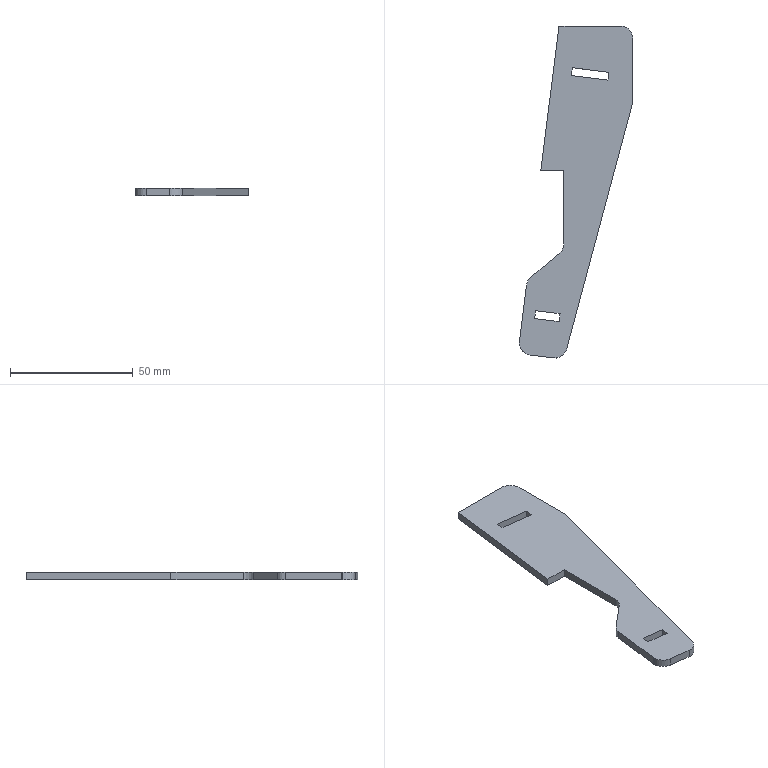Part | SolidWorks | features FlatPattern 1, SMBaseFlange 1, SheetMetal 1 | 1 solid | 26 faces | box 46.127 x 135.184 x 3.2 mm | volume 10243 mm3 | plane 19 | cylinder 7 | commonest cylinder face diameters 10 x7
STEP:
#1=CARTESIAN_POINT('',(-122.572,-320.969,3.2));
#2=VERTEX_POINT('',#1);
#3=CARTESIAN_POINT('',(-118.193,-325.93,3.2));
#4=VERTEX_POINT('',#3);
#5=CARTESIAN_POINT('',(-117.572,-320.969,3.2));
#6=DIRECTION('',(0.,0.,1.));
#7=DIRECTION('',(1.,0.,0.));
#8=AXIS2_PLACEMENT_3D('',#5,#6,#7);
#9=CIRCLE('',#8,5.);
#10=EDGE_CURVE('',#2,#4,#9,.T.);
#11=ORIENTED_EDGE('',*,*,#10,.F.);
#12=CARTESIAN_POINT('',(-122.572,-320.969,0.));
#13=VERTEX_POINT('',#12);
#14=CARTESIAN_POINT('',(-122.572,-320.969,3.2));
#15=DIRECTION('',(0.,0.,-1.));
#16=VECTOR('',#15,1000.);
#17=LINE('',#14,#16);
#18=EDGE_CURVE('',#2,#13,#17,.T.);
#19=ORIENTED_EDGE('',*,*,#18,.T.);
#20=CARTESIAN_POINT('',(-118.193,-325.93,0.));
#21=VERTEX_POINT('',#20);
#22=CARTESIAN_POINT('',(-117.572,-320.969,0.));
#23=DIRECTION('',(0.,0.,1.));
#24=DIRECTION('',(1.,0.,0.));
#25=AXIS2_PLACEMENT_3D('',#22,#23,#24);
#26=CIRCLE('',#25,5.);
#27=EDGE_CURVE('',#13,#21,#26,.T.);
#28=ORIENTED_EDGE('',*,*,#27,.T.);
#29=CARTESIAN_POINT('',(-118.193,-325.93,3.2));
#30=DIRECTION('',(0.,0.,-1.));
#31=VECTOR('',#30,1000.);
#32=LINE('',#29,#31);
#33=EDGE_CURVE('',#4,#21,#32,.T.);
#34=ORIENTED_EDGE('',*,*,#33,.F.);
#35=EDGE_LOOP('',(#11,#19,#28,#34));
#36=FACE_OUTER_BOUND('',#35,.T.);
#37=CARTESIAN_POINT('',(-117.572,-320.969,3.2));
#38=DIRECTION('',(0.,0.,-1.));
#39=DIRECTION('',(-1.,0.,0.));
#40=AXIS2_PLACEMENT_3D('',#37,#38,#39);
#41=CYLINDRICAL_SURFACE('',#40,5.);
#42=ADVANCED_FACE('',(#36),#41,.T.);
#43=CARTESIAN_POINT('',(-86.131,-210.824,3.2));
#44=VERTEX_POINT('',#43);
#45=CARTESIAN_POINT('',(-101.015,-208.958,3.2));
#46=VERTEX_POINT('',#45);
#47=CARTESIAN_POINT('',(-101.015,-208.958,3.2));
#48=DIRECTION('',(-0.9922,0.1243,0.));
#49=VECTOR('',#48,1000.);
#50=LINE('',#47,#49);
#51=EDGE_CURVE('',#44,#46,#50,.T.);
#52=ORIENTED_EDGE('',*,*,#51,.F.);
#53=CARTESIAN_POINT('',(-86.529,-213.999,3.2));
#54=VERTEX_POINT('',#53);
#55=CARTESIAN_POINT('',(-86.131,-210.824,3.2));
#56=DIRECTION('',(0.1243,0.9922,0.));
#57=VECTOR('',#56,1000.);
#58=LINE('',#55,#57);
#59=EDGE_CURVE('',#54,#44,#58,.T.);
#60=ORIENTED_EDGE('',*,*,#59,.F.);
#61=CARTESIAN_POINT('',(-101.413,-212.134,3.2));
#62=VERTEX_POINT('',#61);
#63=CARTESIAN_POINT('',(-86.529,-213.999,3.2));
#64=DIRECTION('',(0.9922,-0.1243,0.));
#65=VECTOR('',#64,1000.);
#66=LINE('',#63,#65);
#67=EDGE_CURVE('',#62,#54,#66,.T.);
#68=ORIENTED_EDGE('',*,*,#67,.F.);
#69=CARTESIAN_POINT('',(-101.413,-212.134,3.2));
#70=DIRECTION('',(-0.1243,-0.9922,0.));
#71=VECTOR('',#70,1000.);
#72=LINE('',#69,#71);
#73=EDGE_CURVE('',#46,#62,#72,.T.);
#74=ORIENTED_EDGE('',*,*,#73,.F.);
#75=EDGE_LOOP('',(#52,#60,#68,#74));
#76=FACE_BOUND('',#75,.T.);
#77=CARTESIAN_POINT('',(-81.445,-191.972,3.2));
#78=VERTEX_POINT('',#77);
#79=CARTESIAN_POINT('',(-106.445,-191.972,3.2));
#80=VERTEX_POINT('',#79);
#81=CARTESIAN_POINT('',(-106.445,-191.972,3.2));
#82=DIRECTION('',(-1.,0.,0.));
#83=VECTOR('',#82,1000.);
#84=LINE('',#81,#83);
#85=EDGE_CURVE('',#78,#80,#84,.T.);
#86=ORIENTED_EDGE('',*,*,#85,.T.);
#87=CARTESIAN_POINT('',(-113.839,-250.972,3.2));
#88=VERTEX_POINT('',#87);
#89=CARTESIAN_POINT('',(-106.445,-191.972,3.2));
#90=DIRECTION('',(-0.1243,-0.9922,0.));
#91=VECTOR('',#90,1000.);
#92=LINE('',#89,#91);
#93=EDGE_CURVE('',#80,#88,#92,.T.);
#94=ORIENTED_EDGE('',*,*,#93,.T.);
#95=CARTESIAN_POINT('',(-104.445,-250.972,3.2));
#96=VERTEX_POINT('',#95);
#97=CARTESIAN_POINT('',(-113.839,-250.972,3.2));
#98=DIRECTION('',(1.,0.,0.));
#99=VECTOR('',#98,1000.);
#100=LINE('',#97,#99);
#101=EDGE_CURVE('',#88,#96,#100,.T.);
#102=ORIENTED_EDGE('',*,*,#101,.T.);
#103=CARTESIAN_POINT('',(-104.445,-280.641,3.2));
#104=VERTEX_POINT('',#103);
#105=CARTESIAN_POINT('',(-104.445,-250.972,3.2));
#106=DIRECTION('',(0.,-1.,0.));
#107=VECTOR('',#106,1000.);
#108=LINE('',#105,#107);
#109=EDGE_CURVE('',#96,#104,#108,.T.);
#110=ORIENTED_EDGE('',*,*,#109,.T.);
#111=CARTESIAN_POINT('',(-106.231,-284.471,3.2));
#112=VERTEX_POINT('',#111);
#113=CARTESIAN_POINT('',(-109.445,-280.641,3.2));
#114=DIRECTION('',(0.,0.,-1.));
#115=DIRECTION('',(1.,0.,0.));
#116=AXIS2_PLACEMENT_3D('',#113,#114,#115);
#117=CIRCLE('',#116,5.);
#118=EDGE_CURVE('',#104,#112,#117,.T.);
#119=ORIENTED_EDGE('',*,*,#118,.T.);
#120=CARTESIAN_POINT('',(-117.921,-294.28,3.2));
#121=VERTEX_POINT('',#120);
#122=CARTESIAN_POINT('',(-117.921,-294.28,3.2));
#123=DIRECTION('',(-0.766,-0.6428,0.));
#124=VECTOR('',#123,1000.);
#125=LINE('',#122,#124);
#126=EDGE_CURVE('',#112,#121,#125,.T.);
#127=ORIENTED_EDGE('',*,*,#126,.T.);
#128=CARTESIAN_POINT('',(-119.668,-297.488,3.2));
#129=VERTEX_POINT('',#128);
#130=CARTESIAN_POINT('',(-114.707,-298.11,3.2));
#131=DIRECTION('',(0.,0.,1.));
#132=DIRECTION('',(1.,0.,0.));
#133=AXIS2_PLACEMENT_3D('',#130,#131,#132);
#134=CIRCLE('',#133,5.);
#135=EDGE_CURVE('',#121,#129,#134,.T.);
#136=ORIENTED_EDGE('',*,*,#135,.T.);
#137=CARTESIAN_POINT('',(-122.533,-320.347,3.2));
#138=VERTEX_POINT('',#137);
#139=CARTESIAN_POINT('',(-119.668,-297.488,3.2));
#140=DIRECTION('',(-0.1243,-0.9922,0.));
#141=VECTOR('',#140,1000.);
#142=LINE('',#139,#141);
#143=EDGE_CURVE('',#129,#138,#142,.T.);
#144=ORIENTED_EDGE('',*,*,#143,.T.);
#145=CARTESIAN_POINT('',(-117.572,-320.969,3.2));
#146=DIRECTION('',(0.,0.,1.));
#147=DIRECTION('',(1.,0.,0.));
#148=AXIS2_PLACEMENT_3D('',#145,#146,#147);
#149=CIRCLE('',#148,5.);
#150=EDGE_CURVE('',#138,#2,#149,.T.);
#151=ORIENTED_EDGE('',*,*,#150,.T.);
#152=ORIENTED_EDGE('',*,*,#10,.T.);
#153=CARTESIAN_POINT('',(-108.717,-327.118,3.2));
#154=VERTEX_POINT('',#153);
#155=CARTESIAN_POINT('',(-118.193,-325.93,3.2));
#156=DIRECTION('',(0.9922,-0.1243,0.));
#157=VECTOR('',#156,1000.);
#158=LINE('',#155,#157);
#159=EDGE_CURVE('',#4,#154,#158,.T.);
#160=ORIENTED_EDGE('',*,*,#159,.T.);
#161=CARTESIAN_POINT('',(-103.266,-323.451,3.2));
#162=VERTEX_POINT('',#161);
#163=CARTESIAN_POINT('',(-108.095,-322.157,3.2));
#164=DIRECTION('',(0.,0.,1.));
#165=DIRECTION('',(-1.,0.,0.));
#166=AXIS2_PLACEMENT_3D('',#163,#164,#165);
#167=CIRCLE('',#166,5.);
#168=EDGE_CURVE('',#154,#162,#167,.T.);
#169=ORIENTED_EDGE('',*,*,#168,.T.);
#170=CARTESIAN_POINT('',(-76.615,-223.99,3.2));
#171=VERTEX_POINT('',#170);
#172=CARTESIAN_POINT('',(-76.615,-223.99,3.2));
#173=DIRECTION('',(0.2588,0.9659,0.));
#174=VECTOR('',#173,1000.);
#175=LINE('',#172,#174);
#176=EDGE_CURVE('',#162,#171,#175,.T.);
#177=ORIENTED_EDGE('',*,*,#176,.T.);
#178=CARTESIAN_POINT('',(-76.445,-222.696,3.2));
#179=VERTEX_POINT('',#178);
#180=CARTESIAN_POINT('',(-81.445,-222.696,3.2));
#181=DIRECTION('',(0.,0.,1.));
#182=DIRECTION('',(-1.,0.,0.));
#183=AXIS2_PLACEMENT_3D('',#180,#181,#182);
#184=CIRCLE('',#183,5.);
#185=EDGE_CURVE('',#171,#179,#184,.T.);
#186=ORIENTED_EDGE('',*,*,#185,.T.);
#187=CARTESIAN_POINT('',(-76.445,-196.972,3.2));
#188=VERTEX_POINT('',#187);
#189=CARTESIAN_POINT('',(-76.445,-196.972,3.2));
#190=DIRECTION('',(0.,1.,0.));
#191=VECTOR('',#190,1000.);
#192=LINE('',#189,#191);
#193=EDGE_CURVE('',#179,#188,#192,.T.);
#194=ORIENTED_EDGE('',*,*,#193,.T.);
#195=CARTESIAN_POINT('',(-81.445,-196.972,3.2));
#196=DIRECTION('',(0.,0.,1.));
#197=DIRECTION('',(-1.,0.,0.));
#198=AXIS2_PLACEMENT_3D('',#195,#196,#197);
#199=CIRCLE('',#198,5.);
#200=EDGE_CURVE('',#188,#78,#199,.T.);
#201=ORIENTED_EDGE('',*,*,#200,.T.);
#202=EDGE_LOOP('',(#86,#94,#102,#110,#119,#127,#136,#144,#151,#152,#160,#169,#177,#186,#194,#201));
#203=FACE_OUTER_BOUND('',#202,.T.);
#204=CARTESIAN_POINT('',(-115.93,-307.872,3.2));
#205=VERTEX_POINT('',#204);
#206=CARTESIAN_POINT('',(-116.328,-311.047,3.2));
#207=VERTEX_POINT('',#206);
#208=CARTESIAN_POINT('',(-116.328,-311.047,3.2));
#209=DIRECTION('',(-0.1243,-0.9922,0.));
#210=VECTOR('',#209,1000.);
#211=LINE('',#208,#210);
#212=EDGE_CURVE('',#205,#207,#211,.T.);
#213=ORIENTED_EDGE('',*,*,#212,.F.);
#214=CARTESIAN_POINT('',(-106.008,-309.115,3.2));
#215=VERTEX_POINT('',#214);
#216=CARTESIAN_POINT('',(-115.93,-307.872,3.2));
#217=DIRECTION('',(-0.9922,0.1243,0.));
#218=VECTOR('',#217,1000.);
#219=LINE('',#216,#218);
#220=EDGE_CURVE('',#215,#205,#219,.T.);
#221=ORIENTED_EDGE('',*,*,#220,.F.);
#222=CARTESIAN_POINT('',(-106.406,-312.29,3.2));
#223=VERTEX_POINT('',#222);
#224=CARTESIAN_POINT('',(-106.008,-309.115,3.2));
#225=DIRECTION('',(0.1243,0.9922,0.));
#226=VECTOR('',#225,1000.);
#227=LINE('',#224,#226);
#228=EDGE_CURVE('',#223,#215,#227,.T.);
#229=ORIENTED_EDGE('',*,*,#228,.F.);
#230=CARTESIAN_POINT('',(-106.406,-312.29,3.2));
#231=DIRECTION('',(0.9922,-0.1243,0.));
#232=VECTOR('',#231,1000.);
#233=LINE('',#230,#232);
#234=EDGE_CURVE('',#207,#223,#233,.T.);
#235=ORIENTED_EDGE('',*,*,#234,.F.);
#236=EDGE_LOOP('',(#213,#221,#229,#235));
#237=FACE_BOUND('',#236,.T.);
#238=CARTESIAN_POINT('',(-81.445,-196.972,3.2));
#239=DIRECTION('',(0.,0.,-1.));
#240=DIRECTION('',(-1.,0.,0.));
#241=AXIS2_PLACEMENT_3D('',#238,#239,#240);
#242=PLANE('',#241);
#243=ADVANCED_FACE('',(#76,#203,#237),#242,.F.);
#244=CARTESIAN_POINT('',(-81.445,-191.972,0.));
#245=VERTEX_POINT('',#244);
#246=CARTESIAN_POINT('',(-106.445,-191.972,0.));
#247=VERTEX_POINT('',#246);
#248=CARTESIAN_POINT('',(-106.445,-191.972,0.));
#249=DIRECTION('',(-1.,0.,0.));
#250=VECTOR('',#249,1000.);
#251=LINE('',#248,#250);
#252=EDGE_CURVE('',#245,#247,#251,.T.);
#253=ORIENTED_EDGE('',*,*,#252,.F.);
#254=CARTESIAN_POINT('',(-76.445,-196.972,0.));
#255=VERTEX_POINT('',#254);
#256=CARTESIAN_POINT('',(-81.445,-196.972,0.));
#257=DIRECTION('',(0.,0.,1.));
#258=DIRECTION('',(-1.,0.,0.));
#259=AXIS2_PLACEMENT_3D('',#256,#257,#258);
#260=CIRCLE('',#259,5.);
#261=EDGE_CURVE('',#255,#245,#260,.T.);
#262=ORIENTED_EDGE('',*,*,#261,.F.);
#263=CARTESIAN_POINT('',(-76.445,-222.696,0.));
#264=VERTEX_POINT('',#263);
#265=CARTESIAN_POINT('',(-76.445,-196.972,0.));
#266=DIRECTION('',(0.,1.,0.));
#267=VECTOR('',#266,1000.);
#268=LINE('',#265,#267);
#269=EDGE_CURVE('',#264,#255,#268,.T.);
#270=ORIENTED_EDGE('',*,*,#269,.F.);
#271=CARTESIAN_POINT('',(-76.615,-223.99,0.));
#272=VERTEX_POINT('',#271);
#273=CARTESIAN_POINT('',(-81.445,-222.696,0.));
#274=DIRECTION('',(0.,0.,1.));
#275=DIRECTION('',(-1.,0.,0.));
#276=AXIS2_PLACEMENT_3D('',#273,#274,#275);
#277=CIRCLE('',#276,5.);
#278=EDGE_CURVE('',#272,#264,#277,.T.);
#279=ORIENTED_EDGE('',*,*,#278,.F.);
#280=CARTESIAN_POINT('',(-103.266,-323.451,0.));
#281=VERTEX_POINT('',#280);
#282=CARTESIAN_POINT('',(-76.615,-223.99,0.));
#283=DIRECTION('',(0.2588,0.9659,0.));
#284=VECTOR('',#283,1000.);
#285=LINE('',#282,#284);
#286=EDGE_CURVE('',#281,#272,#285,.T.);
#287=ORIENTED_EDGE('',*,*,#286,.F.);
#288=CARTESIAN_POINT('',(-108.717,-327.118,0.));
#289=VERTEX_POINT('',#288);
#290=CARTESIAN_POINT('',(-108.095,-322.157,0.));
#291=DIRECTION('',(0.,0.,1.));
#292=DIRECTION('',(-1.,0.,0.));
#293=AXIS2_PLACEMENT_3D('',#290,#291,#292);
#294=CIRCLE('',#293,5.);
#295=EDGE_CURVE('',#289,#281,#294,.T.);
#296=ORIENTED_EDGE('',*,*,#295,.F.);
#297=CARTESIAN_POINT('',(-118.193,-325.93,0.));
#298=DIRECTION('',(0.9922,-0.1243,0.));
#299=VECTOR('',#298,1000.);
#300=LINE('',#297,#299);
#301=EDGE_CURVE('',#21,#289,#300,.T.);
#302=ORIENTED_EDGE('',*,*,#301,.F.);
#303=ORIENTED_EDGE('',*,*,#27,.F.);
#304=CARTESIAN_POINT('',(-122.533,-320.347,0.));
#305=VERTEX_POINT('',#304);
#306=CARTESIAN_POINT('',(-117.572,-320.969,0.));
#307=DIRECTION('',(0.,0.,1.));
#308=DIRECTION('',(1.,0.,0.));
#309=AXIS2_PLACEMENT_3D('',#306,#307,#308);
#310=CIRCLE('',#309,5.);
#311=EDGE_CURVE('',#305,#13,#310,.T.);
#312=ORIENTED_EDGE('',*,*,#311,.F.);
#313=CARTESIAN_POINT('',(-119.668,-297.488,0.));
#314=VERTEX_POINT('',#313);
#315=CARTESIAN_POINT('',(-119.668,-297.488,0.));
#316=DIRECTION('',(-0.1243,-0.9922,0.));
#317=VECTOR('',#316,1000.);
#318=LINE('',#315,#317);
#319=EDGE_CURVE('',#314,#305,#318,.T.);
#320=ORIENTED_EDGE('',*,*,#319,.F.);
#321=CARTESIAN_POINT('',(-117.921,-294.28,0.));
#322=VERTEX_POINT('',#321);
#323=CARTESIAN_POINT('',(-114.707,-298.11,0.));
#324=DIRECTION('',(0.,0.,1.));
#325=DIRECTION('',(1.,0.,0.));
#326=AXIS2_PLACEMENT_3D('',#323,#324,#325);
#327=CIRCLE('',#326,5.);
#328=EDGE_CURVE('',#322,#314,#327,.T.);
#329=ORIENTED_EDGE('',*,*,#328,.F.);
#330=CARTESIAN_POINT('',(-106.231,-284.471,0.));
#331=VERTEX_POINT('',#330);
#332=CARTESIAN_POINT('',(-117.921,-294.28,0.));
#333=DIRECTION('',(-0.766,-0.6428,0.));
#334=VECTOR('',#333,1000.);
#335=LINE('',#332,#334);
#336=EDGE_CURVE('',#331,#322,#335,.T.);
#337=ORIENTED_EDGE('',*,*,#336,.F.);
#338=CARTESIAN_POINT('',(-104.445,-280.641,0.));
#339=VERTEX_POINT('',#338);
#340=CARTESIAN_POINT('',(-109.445,-280.641,0.));
#341=DIRECTION('',(0.,0.,-1.));
#342=DIRECTION('',(1.,0.,0.));
#343=AXIS2_PLACEMENT_3D('',#340,#341,#342);
#344=CIRCLE('',#343,5.);
#345=EDGE_CURVE('',#339,#331,#344,.T.);
#346=ORIENTED_EDGE('',*,*,#345,.F.);
#347=CARTESIAN_POINT('',(-104.445,-250.972,0.));
#348=VERTEX_POINT('',#347);
#349=CARTESIAN_POINT('',(-104.445,-250.972,0.));
#350=DIRECTION('',(0.,-1.,0.));
#351=VECTOR('',#350,1000.);
#352=LINE('',#349,#351);
#353=EDGE_CURVE('',#348,#339,#352,.T.);
#354=ORIENTED_EDGE('',*,*,#353,.F.);
#355=CARTESIAN_POINT('',(-113.839,-250.972,0.));
#356=VERTEX_POINT('',#355);
#357=CARTESIAN_POINT('',(-113.839,-250.972,0.));
#358=DIRECTION('',(1.,0.,0.));
#359=VECTOR('',#358,1000.);
#360=LINE('',#357,#359);
#361=EDGE_CURVE('',#356,#348,#360,.T.);
#362=ORIENTED_EDGE('',*,*,#361,.F.);
#363=CARTESIAN_POINT('',(-106.445,-191.972,0.));
#364=DIRECTION('',(-0.1243,-0.9922,0.));
#365=VECTOR('',#364,1000.);
#366=LINE('',#363,#365);
#367=EDGE_CURVE('',#247,#356,#366,.T.);
#368=ORIENTED_EDGE('',*,*,#367,.F.);
#369=EDGE_LOOP('',(#253,#262,#270,#279,#287,#296,#302,#303,#312,#320,#329,#337,#346,#354,#362,#368));
#370=FACE_OUTER_BOUND('',#369,.T.);
#371=CARTESIAN_POINT('',(-86.529,-213.999,0.));
#372=VERTEX_POINT('',#371);
#373=CARTESIAN_POINT('',(-86.131,-210.824,0.));
#374=VERTEX_POINT('',#373);
#375=CARTESIAN_POINT('',(-86.131,-210.824,0.));
#376=DIRECTION('',(0.1243,0.9922,0.));
#377=VECTOR('',#376,1000.);
#378=LINE('',#375,#377);
#379=EDGE_CURVE('',#372,#374,#378,.T.);
#380=ORIENTED_EDGE('',*,*,#379,.T.);
#381=CARTESIAN_POINT('',(-101.015,-208.958,0.));
#382=VERTEX_POINT('',#381);
#383=CARTESIAN_POINT('',(-101.015,-208.958,0.));
#384=DIRECTION('',(-0.9922,0.1243,0.));
#385=VECTOR('',#384,1000.);
#386=LINE('',#383,#385);
#387=EDGE_CURVE('',#374,#382,#386,.T.);
#388=ORIENTED_EDGE('',*,*,#387,.T.);
#389=CARTESIAN_POINT('',(-101.413,-212.134,0.));
#390=VERTEX_POINT('',#389);
#391=CARTESIAN_POINT('',(-101.413,-212.134,0.));
#392=DIRECTION('',(-0.1243,-0.9922,0.));
#393=VECTOR('',#392,1000.);
#394=LINE('',#391,#393);
#395=EDGE_CURVE('',#382,#390,#394,.T.);
#396=ORIENTED_EDGE('',*,*,#395,.T.);
#397=CARTESIAN_POINT('',(-86.529,-213.999,0.));
#398=DIRECTION('',(0.9922,-0.1243,0.));
#399=VECTOR('',#398,1000.);
#400=LINE('',#397,#399);
#401=EDGE_CURVE('',#390,#372,#400,.T.);
#402=ORIENTED_EDGE('',*,*,#401,.T.);
#403=EDGE_LOOP('',(#380,#388,#396,#402));
#404=FACE_BOUND('',#403,.T.);
#405=CARTESIAN_POINT('',(-106.008,-309.115,0.));
#406=VERTEX_POINT('',#405);
#407=CARTESIAN_POINT('',(-115.93,-307.872,0.));
#408=VERTEX_POINT('',#407);
#409=CARTESIAN_POINT('',(-115.93,-307.872,0.));
#410=DIRECTION('',(-0.9922,0.1243,0.));
#411=VECTOR('',#410,1000.);
#412=LINE('',#409,#411);
#413=EDGE_CURVE('',#406,#408,#412,.T.);
#414=ORIENTED_EDGE('',*,*,#413,.T.);
#415=CARTESIAN_POINT('',(-116.328,-311.047,0.));
#416=VERTEX_POINT('',#415);
#417=CARTESIAN_POINT('',(-116.328,-311.047,0.));
#418=DIRECTION('',(-0.1243,-0.9922,0.));
#419=VECTOR('',#418,1000.);
#420=LINE('',#417,#419);
#421=EDGE_CURVE('',#408,#416,#420,.T.);
#422=ORIENTED_EDGE('',*,*,#421,.T.);
#423=CARTESIAN_POINT('',(-106.406,-312.29,0.));
#424=VERTEX_POINT('',#423);
#425=CARTESIAN_POINT('',(-106.406,-312.29,0.));
#426=DIRECTION('',(0.9922,-0.1243,0.));
#427=VECTOR('',#426,1000.);
#428=LINE('',#425,#427);
#429=EDGE_CURVE('',#416,#424,#428,.T.);
#430=ORIENTED_EDGE('',*,*,#429,.T.);
#431=CARTESIAN_POINT('',(-106.008,-309.115,0.));
#432=DIRECTION('',(0.1243,0.9922,0.));
#433=VECTOR('',#432,1000.);
#434=LINE('',#431,#433);
#435=EDGE_CURVE('',#424,#406,#434,.T.);
#436=ORIENTED_EDGE('',*,*,#435,.T.);
#437=EDGE_LOOP('',(#414,#422,#430,#436));
#438=FACE_BOUND('',#437,.T.);
#439=CARTESIAN_POINT('',(-81.445,-196.972,0.));
#440=DIRECTION('',(0.,0.,-1.));
#441=DIRECTION('',(-1.,0.,0.));
#442=AXIS2_PLACEMENT_3D('',#439,#440,#441);
#443=PLANE('',#442);
#444=ADVANCED_FACE('',(#370,#404,#438),#443,.T.);
#445=ORIENTED_EDGE('',*,*,#252,.T.);
#446=CARTESIAN_POINT('',(-106.445,-191.972,3.2));
#447=DIRECTION('',(0.,0.,-1.));
#448=VECTOR('',#447,1000.);
#449=LINE('',#446,#448);
#450=EDGE_CURVE('',#80,#247,#449,.T.);
#451=ORIENTED_EDGE('',*,*,#450,.F.);
#452=ORIENTED_EDGE('',*,*,#85,.F.);
#453=CARTESIAN_POINT('',(-81.445,-191.972,3.2));
#454=DIRECTION('',(0.,0.,-1.));
#455=VECTOR('',#454,1000.);
#456=LINE('',#453,#455);
#457=EDGE_CURVE('',#78,#245,#456,.T.);
#458=ORIENTED_EDGE('',*,*,#457,.T.);
#459=EDGE_LOOP('',(#445,#451,#452,#458));
#460=FACE_OUTER_BOUND('',#459,.T.);
#461=CARTESIAN_POINT('',(-106.445,-191.972,3.2));
#462=DIRECTION('',(0.,-1.,0.));
#463=DIRECTION('',(0.,0.,-1.));
#464=AXIS2_PLACEMENT_3D('',#461,#462,#463);
#465=PLANE('',#464);
#466=ADVANCED_FACE('',(#460),#465,.F.);
#467=ORIENTED_EDGE('',*,*,#367,.T.);
#468=CARTESIAN_POINT('',(-113.839,-250.972,3.2));
#469=DIRECTION('',(0.,0.,-1.));
#470=VECTOR('',#469,1000.);
#471=LINE('',#468,#470);
#472=EDGE_CURVE('',#88,#356,#471,.T.);
#473=ORIENTED_EDGE('',*,*,#472,.F.);
#474=ORIENTED_EDGE('',*,*,#93,.F.);
#475=ORIENTED_EDGE('',*,*,#450,.T.);
#476=EDGE_LOOP('',(#467,#473,#474,#475));
#477=FACE_OUTER_BOUND('',#476,.T.);
#478=CARTESIAN_POINT('',(-106.445,-191.972,3.2));
#479=DIRECTION('',(0.9922,-0.1243,0.));
#480=DIRECTION('',(0.1243,0.9922,0.));
#481=AXIS2_PLACEMENT_3D('',#478,#479,#480);
#482=PLANE('',#481);
#483=ADVANCED_FACE('',(#477),#482,.F.);
#484=ORIENTED_EDGE('',*,*,#361,.T.);
#485=CARTESIAN_POINT('',(-104.445,-250.972,3.2));
#486=DIRECTION('',(0.,0.,-1.));
#487=VECTOR('',#486,1000.);
#488=LINE('',#485,#487);
#489=EDGE_CURVE('',#96,#348,#488,.T.);
#490=ORIENTED_EDGE('',*,*,#489,.F.);
#491=ORIENTED_EDGE('',*,*,#101,.F.);
#492=ORIENTED_EDGE('',*,*,#472,.T.);
#493=EDGE_LOOP('',(#484,#490,#491,#492));
#494=FACE_OUTER_BOUND('',#493,.T.);
#495=CARTESIAN_POINT('',(-113.839,-250.972,3.2));
#496=DIRECTION('',(0.,1.,0.));
#497=DIRECTION('',(0.,0.,1.));
#498=AXIS2_PLACEMENT_3D('',#495,#496,#497);
#499=PLANE('',#498);
#500=ADVANCED_FACE('',(#494),#499,.F.);
#501=ORIENTED_EDGE('',*,*,#353,.T.);
#502=CARTESIAN_POINT('',(-104.445,-280.641,3.2));
#503=DIRECTION('',(0.,0.,-1.));
#504=VECTOR('',#503,1000.);
#505=LINE('',#502,#504);
#506=EDGE_CURVE('',#104,#339,#505,.T.);
#507=ORIENTED_EDGE('',*,*,#506,.F.);
#508=ORIENTED_EDGE('',*,*,#109,.F.);
#509=ORIENTED_EDGE('',*,*,#489,.T.);
#510=EDGE_LOOP('',(#501,#507,#508,#509));
#511=FACE_OUTER_BOUND('',#510,.T.);
#512=CARTESIAN_POINT('',(-104.445,-250.972,3.2));
#513=DIRECTION('',(1.,0.,0.));
#514=DIRECTION('',(0.,1.,0.));
#515=AXIS2_PLACEMENT_3D('',#512,#513,#514);
#516=PLANE('',#515);
#517=ADVANCED_FACE('',(#511),#516,.F.);
#518=ORIENTED_EDGE('',*,*,#345,.T.);
#519=CARTESIAN_POINT('',(-106.231,-284.471,3.2));
#520=DIRECTION('',(0.,0.,-1.));
#521=VECTOR('',#520,1000.);
#522=LINE('',#519,#521);
#523=EDGE_CURVE('',#112,#331,#522,.T.);
#524=ORIENTED_EDGE('',*,*,#523,.F.);
#525=ORIENTED_EDGE('',*,*,#118,.F.);
#526=ORIENTED_EDGE('',*,*,#506,.T.);
#527=EDGE_LOOP('',(#518,#524,#525,#526));
#528=FACE_OUTER_BOUND('',#527,.T.);
#529=CARTESIAN_POINT('',(-109.445,-280.641,3.2));
#530=DIRECTION('',(0.,0.,-1.));
#531=DIRECTION('',(-1.,0.,0.));
#532=AXIS2_PLACEMENT_3D('',#529,#530,#531);
#533=CYLINDRICAL_SURFACE('',#532,5.);
#534=ADVANCED_FACE('',(#528),#533,.F.);
#535=ORIENTED_EDGE('',*,*,#336,.T.);
#536=CARTESIAN_POINT('',(-117.921,-294.28,3.2));
#537=DIRECTION('',(0.,0.,-1.));
#538=VECTOR('',#537,1000.);
#539=LINE('',#536,#538);
#540=EDGE_CURVE('',#121,#322,#539,.T.);
#541=ORIENTED_EDGE('',*,*,#540,.F.);
#542=ORIENTED_EDGE('',*,*,#126,.F.);
#543=ORIENTED_EDGE('',*,*,#523,.T.);
#544=EDGE_LOOP('',(#535,#541,#542,#543));
#545=FACE_OUTER_BOUND('',#544,.T.);
#546=CARTESIAN_POINT('',(-117.921,-294.28,3.2));
#547=DIRECTION('',(0.6428,-0.766,0.));
#548=DIRECTION('',(0.766,0.6428,0.));
#549=AXIS2_PLACEMENT_3D('',#546,#547,#548);
#550=PLANE('',#549);
#551=ADVANCED_FACE('',(#545),#550,.F.);
#552=ORIENTED_EDGE('',*,*,#328,.T.);
#553=CARTESIAN_POINT('',(-119.668,-297.488,3.2));
#554=DIRECTION('',(0.,0.,-1.));
#555=VECTOR('',#554,1000.);
#556=LINE('',#553,#555);
#557=EDGE_CURVE('',#129,#314,#556,.T.);
#558=ORIENTED_EDGE('',*,*,#557,.F.);
#559=ORIENTED_EDGE('',*,*,#135,.F.);
#560=ORIENTED_EDGE('',*,*,#540,.T.);
#561=EDGE_LOOP('',(#552,#558,#559,#560));
#562=FACE_OUTER_BOUND('',#561,.T.);
#563=CARTESIAN_POINT('',(-114.707,-298.11,3.2));
#564=DIRECTION('',(0.,0.,-1.));
#565=DIRECTION('',(-1.,0.,0.));
#566=AXIS2_PLACEMENT_3D('',#563,#564,#565);
#567=CYLINDRICAL_SURFACE('',#566,5.);
#568=ADVANCED_FACE('',(#562),#567,.T.);
#569=ORIENTED_EDGE('',*,*,#319,.T.);
#570=CARTESIAN_POINT('',(-122.533,-320.347,3.2));
#571=DIRECTION('',(0.,0.,-1.));
#572=VECTOR('',#571,1000.);
#573=LINE('',#570,#572);
#574=EDGE_CURVE('',#138,#305,#573,.T.);
#575=ORIENTED_EDGE('',*,*,#574,.F.);
#576=ORIENTED_EDGE('',*,*,#143,.F.);
#577=ORIENTED_EDGE('',*,*,#557,.T.);
#578=EDGE_LOOP('',(#569,#575,#576,#577));
#579=FACE_OUTER_BOUND('',#578,.T.);
#580=CARTESIAN_POINT('',(-119.668,-297.488,3.2));
#581=DIRECTION('',(0.9922,-0.1243,0.));
#582=DIRECTION('',(0.1243,0.9922,0.));
#583=AXIS2_PLACEMENT_3D('',#580,#581,#582);
#584=PLANE('',#583);
#585=ADVANCED_FACE('',(#579),#584,.F.);
#586=ORIENTED_EDGE('',*,*,#18,.F.);
#587=ORIENTED_EDGE('',*,*,#150,.F.);
#588=ORIENTED_EDGE('',*,*,#574,.T.);
#589=ORIENTED_EDGE('',*,*,#311,.T.);
#590=EDGE_LOOP('',(#586,#587,#588,#589));
#591=FACE_OUTER_BOUND('',#590,.T.);
#592=CARTESIAN_POINT('',(-117.572,-320.969,3.2));
#593=DIRECTION('',(0.,0.,-1.));
#594=DIRECTION('',(-1.,0.,0.));
#595=AXIS2_PLACEMENT_3D('',#592,#593,#594);
#596=CYLINDRICAL_SURFACE('',#595,5.);
#597=ADVANCED_FACE('',(#591),#596,.T.);
#598=ORIENTED_EDGE('',*,*,#301,.T.);
#599=CARTESIAN_POINT('',(-108.717,-327.118,3.2));
#600=DIRECTION('',(0.,0.,-1.));
#601=VECTOR('',#600,1000.);
#602=LINE('',#599,#601);
#603=EDGE_CURVE('',#154,#289,#602,.T.);
#604=ORIENTED_EDGE('',*,*,#603,.F.);
#605=ORIENTED_EDGE('',*,*,#159,.F.);
#606=ORIENTED_EDGE('',*,*,#33,.T.);
#607=EDGE_LOOP('',(#598,#604,#605,#606));
#608=FACE_OUTER_BOUND('',#607,.T.);
#609=CARTESIAN_POINT('',(-118.193,-325.93,3.2));
#610=DIRECTION('',(0.1243,0.9922,0.));
#611=DIRECTION('',(-0.9922,0.1243,0.));
#612=AXIS2_PLACEMENT_3D('',#609,#610,#611);
#613=PLANE('',#612);
#614=ADVANCED_FACE('',(#608),#613,.F.);
#615=ORIENTED_EDGE('',*,*,#295,.T.);
#616=CARTESIAN_POINT('',(-103.266,-323.451,3.2));
#617=DIRECTION('',(0.,0.,-1.));
#618=VECTOR('',#617,1000.);
#619=LINE('',#616,#618);
#620=EDGE_CURVE('',#162,#281,#619,.T.);
#621=ORIENTED_EDGE('',*,*,#620,.F.);
#622=ORIENTED_EDGE('',*,*,#168,.F.);
#623=ORIENTED_EDGE('',*,*,#603,.T.);
#624=EDGE_LOOP('',(#615,#621,#622,#623));
#625=FACE_OUTER_BOUND('',#624,.T.);
#626=CARTESIAN_POINT('',(-108.095,-322.157,3.2));
#627=DIRECTION('',(0.,0.,-1.));
#628=DIRECTION('',(-1.,0.,0.));
#629=AXIS2_PLACEMENT_3D('',#626,#627,#628);
#630=CYLINDRICAL_SURFACE('',#629,5.);
#631=ADVANCED_FACE('',(#625),#630,.T.);
#632=ORIENTED_EDGE('',*,*,#286,.T.);
#633=CARTESIAN_POINT('',(-76.615,-223.99,3.2));
#634=DIRECTION('',(0.,0.,-1.));
#635=VECTOR('',#634,1000.);
#636=LINE('',#633,#635);
#637=EDGE_CURVE('',#171,#272,#636,.T.);
#638=ORIENTED_EDGE('',*,*,#637,.F.);
#639=ORIENTED_EDGE('',*,*,#176,.F.);
#640=ORIENTED_EDGE('',*,*,#620,.T.);
#641=EDGE_LOOP('',(#632,#638,#639,#640));
#642=FACE_OUTER_BOUND('',#641,.T.);
#643=CARTESIAN_POINT('',(-76.615,-223.99,3.2));
#644=DIRECTION('',(-0.9659,0.2588,0.));
#645=DIRECTION('',(-0.2588,-0.9659,0.));
#646=AXIS2_PLACEMENT_3D('',#643,#644,#645);
#647=PLANE('',#646);
#648=ADVANCED_FACE('',(#642),#647,.F.);
#649=ORIENTED_EDGE('',*,*,#278,.T.);
#650=CARTESIAN_POINT('',(-76.445,-222.696,3.2));
#651=DIRECTION('',(0.,0.,-1.));
#652=VECTOR('',#651,1000.);
#653=LINE('',#650,#652);
#654=EDGE_CURVE('',#179,#264,#653,.T.);
#655=ORIENTED_EDGE('',*,*,#654,.F.);
#656=ORIENTED_EDGE('',*,*,#185,.F.);
#657=ORIENTED_EDGE('',*,*,#637,.T.);
#658=EDGE_LOOP('',(#649,#655,#656,#657));
#659=FACE_OUTER_BOUND('',#658,.T.);
#660=CARTESIAN_POINT('',(-81.445,-222.696,3.2));
#661=DIRECTION('',(0.,0.,-1.));
#662=DIRECTION('',(-1.,0.,0.));
#663=AXIS2_PLACEMENT_3D('',#660,#661,#662);
#664=CYLINDRICAL_SURFACE('',#663,5.);
#665=ADVANCED_FACE('',(#659),#664,.T.);
#666=ORIENTED_EDGE('',*,*,#269,.T.);
#667=CARTESIAN_POINT('',(-76.445,-196.972,3.2));
#668=DIRECTION('',(0.,0.,-1.));
#669=VECTOR('',#668,1000.);
#670=LINE('',#667,#669);
#671=EDGE_CURVE('',#188,#255,#670,.T.);
#672=ORIENTED_EDGE('',*,*,#671,.F.);
#673=ORIENTED_EDGE('',*,*,#193,.F.);
#674=ORIENTED_EDGE('',*,*,#654,.T.);
#675=EDGE_LOOP('',(#666,#672,#673,#674));
#676=FACE_OUTER_BOUND('',#675,.T.);
#677=CARTESIAN_POINT('',(-76.445,-196.972,3.2));
#678=DIRECTION('',(-1.,0.,0.));
#679=DIRECTION('',(0.,0.,1.));
#680=AXIS2_PLACEMENT_3D('',#677,#678,#679);
#681=PLANE('',#680);
#682=ADVANCED_FACE('',(#676),#681,.F.);
#683=ORIENTED_EDGE('',*,*,#261,.T.);
#684=ORIENTED_EDGE('',*,*,#457,.F.);
#685=ORIENTED_EDGE('',*,*,#200,.F.);
#686=ORIENTED_EDGE('',*,*,#671,.T.);
#687=EDGE_LOOP('',(#683,#684,#685,#686));
#688=FACE_OUTER_BOUND('',#687,.T.);
#689=CARTESIAN_POINT('',(-81.445,-196.972,3.2));
#690=DIRECTION('',(0.,0.,-1.));
#691=DIRECTION('',(-1.,0.,0.));
#692=AXIS2_PLACEMENT_3D('',#689,#690,#691);
#693=CYLINDRICAL_SURFACE('',#692,5.);
#694=ADVANCED_FACE('',(#688),#693,.T.);
#695=ORIENTED_EDGE('',*,*,#387,.F.);
#696=CARTESIAN_POINT('',(-86.131,-210.824,3.2));
#697=DIRECTION('',(0.,0.,-1.));
#698=VECTOR('',#697,1000.);
#699=LINE('',#696,#698);
#700=EDGE_CURVE('',#44,#374,#699,.T.);
#701=ORIENTED_EDGE('',*,*,#700,.F.);
#702=ORIENTED_EDGE('',*,*,#51,.T.);
#703=CARTESIAN_POINT('',(-101.015,-208.958,3.2));
#704=DIRECTION('',(0.,0.,-1.));
#705=VECTOR('',#704,1000.);
#706=LINE('',#703,#705);
#707=EDGE_CURVE('',#46,#382,#706,.T.);
#708=ORIENTED_EDGE('',*,*,#707,.T.);
#709=EDGE_LOOP('',(#695,#701,#702,#708));
#710=FACE_OUTER_BOUND('',#709,.T.);
#711=CARTESIAN_POINT('',(-101.015,-208.958,3.2));
#712=DIRECTION('',(-0.1243,-0.9922,0.));
#713=DIRECTION('',(0.9922,-0.1243,0.));
#714=AXIS2_PLACEMENT_3D('',#711,#712,#713);
#715=PLANE('',#714);
#716=ADVANCED_FACE('',(#710),#715,.T.);
#717=ORIENTED_EDGE('',*,*,#395,.F.);
#718=ORIENTED_EDGE('',*,*,#707,.F.);
#719=ORIENTED_EDGE('',*,*,#73,.T.);
#720=CARTESIAN_POINT('',(-101.413,-212.134,3.2));
#721=DIRECTION('',(0.,0.,-1.));
#722=VECTOR('',#721,1000.);
#723=LINE('',#720,#722);
#724=EDGE_CURVE('',#62,#390,#723,.T.);
#725=ORIENTED_EDGE('',*,*,#724,.T.);
#726=EDGE_LOOP('',(#717,#718,#719,#725));
#727=FACE_OUTER_BOUND('',#726,.T.);
#728=CARTESIAN_POINT('',(-101.413,-212.134,3.2));
#729=DIRECTION('',(0.9922,-0.1243,0.));
#730=DIRECTION('',(0.1243,0.9922,0.));
#731=AXIS2_PLACEMENT_3D('',#728,#729,#730);
#732=PLANE('',#731);
#733=ADVANCED_FACE('',(#727),#732,.T.);
#734=ORIENTED_EDGE('',*,*,#401,.F.);
#735=ORIENTED_EDGE('',*,*,#724,.F.);
#736=ORIENTED_EDGE('',*,*,#67,.T.);
#737=CARTESIAN_POINT('',(-86.529,-213.999,3.2));
#738=DIRECTION('',(0.,0.,-1.));
#739=VECTOR('',#738,1000.);
#740=LINE('',#737,#739);
#741=EDGE_CURVE('',#54,#372,#740,.T.);
#742=ORIENTED_EDGE('',*,*,#741,.T.);
#743=EDGE_LOOP('',(#734,#735,#736,#742));
#744=FACE_OUTER_BOUND('',#743,.T.);
#745=CARTESIAN_POINT('',(-86.529,-213.999,3.2));
#746=DIRECTION('',(0.1243,0.9922,0.));
#747=DIRECTION('',(-0.9922,0.1243,0.));
#748=AXIS2_PLACEMENT_3D('',#745,#746,#747);
#749=PLANE('',#748);
#750=ADVANCED_FACE('',(#744),#749,.T.);
#751=ORIENTED_EDGE('',*,*,#379,.F.);
#752=ORIENTED_EDGE('',*,*,#741,.F.);
#753=ORIENTED_EDGE('',*,*,#59,.T.);
#754=ORIENTED_EDGE('',*,*,#700,.T.);
#755=EDGE_LOOP('',(#751,#752,#753,#754));
#756=FACE_OUTER_BOUND('',#755,.T.);
#757=CARTESIAN_POINT('',(-86.131,-210.824,3.2));
#758=DIRECTION('',(-0.9922,0.1243,0.));
#759=DIRECTION('',(-0.1243,-0.9922,0.));
#760=AXIS2_PLACEMENT_3D('',#757,#758,#759);
#761=PLANE('',#760);
#762=ADVANCED_FACE('',(#756),#761,.T.);
#763=ORIENTED_EDGE('',*,*,#421,.F.);
#764=CARTESIAN_POINT('',(-115.93,-307.872,3.2));
#765=DIRECTION('',(0.,0.,-1.));
#766=VECTOR('',#765,1000.);
#767=LINE('',#764,#766);
#768=EDGE_CURVE('',#205,#408,#767,.T.);
#769=ORIENTED_EDGE('',*,*,#768,.F.);
#770=ORIENTED_EDGE('',*,*,#212,.T.);
#771=CARTESIAN_POINT('',(-116.328,-311.047,3.2));
#772=DIRECTION('',(0.,0.,-1.));
#773=VECTOR('',#772,1000.);
#774=LINE('',#771,#773);
#775=EDGE_CURVE('',#207,#416,#774,.T.);
#776=ORIENTED_EDGE('',*,*,#775,.T.);
#777=EDGE_LOOP('',(#763,#769,#770,#776));
#778=FACE_OUTER_BOUND('',#777,.T.);
#779=CARTESIAN_POINT('',(-116.328,-311.047,3.2));
#780=DIRECTION('',(0.9922,-0.1243,0.));
#781=DIRECTION('',(0.1243,0.9922,0.));
#782=AXIS2_PLACEMENT_3D('',#779,#780,#781);
#783=PLANE('',#782);
#784=ADVANCED_FACE('',(#778),#783,.T.);
#785=ORIENTED_EDGE('',*,*,#429,.F.);
#786=ORIENTED_EDGE('',*,*,#775,.F.);
#787=ORIENTED_EDGE('',*,*,#234,.T.);
#788=CARTESIAN_POINT('',(-106.406,-312.29,3.2));
#789=DIRECTION('',(0.,0.,-1.));
#790=VECTOR('',#789,1000.);
#791=LINE('',#788,#790);
#792=EDGE_CURVE('',#223,#424,#791,.T.);
#793=ORIENTED_EDGE('',*,*,#792,.T.);
#794=EDGE_LOOP('',(#785,#786,#787,#793));
#795=FACE_OUTER_BOUND('',#794,.T.);
#796=CARTESIAN_POINT('',(-106.406,-312.29,3.2));
#797=DIRECTION('',(0.1243,0.9922,0.));
#798=DIRECTION('',(-0.9922,0.1243,0.));
#799=AXIS2_PLACEMENT_3D('',#796,#797,#798);
#800=PLANE('',#799);
#801=ADVANCED_FACE('',(#795),#800,.T.);
#802=ORIENTED_EDGE('',*,*,#435,.F.);
#803=ORIENTED_EDGE('',*,*,#792,.F.);
#804=ORIENTED_EDGE('',*,*,#228,.T.);
#805=CARTESIAN_POINT('',(-106.008,-309.115,3.2));
#806=DIRECTION('',(0.,0.,-1.));
#807=VECTOR('',#806,1000.);
#808=LINE('',#805,#807);
#809=EDGE_CURVE('',#215,#406,#808,.T.);
#810=ORIENTED_EDGE('',*,*,#809,.T.);
#811=EDGE_LOOP('',(#802,#803,#804,#810));
#812=FACE_OUTER_BOUND('',#811,.T.);
#813=CARTESIAN_POINT('',(-106.008,-309.115,3.2));
#814=DIRECTION('',(-0.9922,0.1243,0.));
#815=DIRECTION('',(-0.1243,-0.9922,0.));
#816=AXIS2_PLACEMENT_3D('',#813,#814,#815);
#817=PLANE('',#816);
#818=ADVANCED_FACE('',(#812),#817,.T.);
#819=ORIENTED_EDGE('',*,*,#413,.F.);
#820=ORIENTED_EDGE('',*,*,#809,.F.);
#821=ORIENTED_EDGE('',*,*,#220,.T.);
#822=ORIENTED_EDGE('',*,*,#768,.T.);
#823=EDGE_LOOP('',(#819,#820,#821,#822));
#824=FACE_OUTER_BOUND('',#823,.T.);
#825=CARTESIAN_POINT('',(-115.93,-307.872,3.2));
#826=DIRECTION('',(-0.1243,-0.9922,0.));
#827=DIRECTION('',(0.9922,-0.1243,0.));
#828=AXIS2_PLACEMENT_3D('',#825,#826,#827);
#829=PLANE('',#828);
#830=ADVANCED_FACE('',(#824),#829,.T.);
#831=CLOSED_SHELL('',(#42,#243,#444,#466,#483,#500,#517,#534,#551,#568,#585,#597,#614,#631,#648,#665,#682,#694,#716,#733,#750,#762,#784,#801,#818,#830));
#832=MANIFOLD_SOLID_BREP('',#831);
#833=CARTESIAN_POINT('',(0.,0.,0.));
#834=DIRECTION('',(0.,0.,1.));
#835=DIRECTION('',(1.,0.,0.));
#836=AXIS2_PLACEMENT_3D('',#833,#834,#835);
#837=(LENGTH_UNIT()NAMED_UNIT(*)SI_UNIT(.MILLI.,.METRE.));
#838=UNCERTAINTY_MEASURE_WITH_UNIT(LENGTH_MEASURE(0.00001),#837,'','');
#839=(NAMED_UNIT(*)PLANE_ANGLE_UNIT()SI_UNIT($,.RADIAN.));
#840=(NAMED_UNIT(*)SI_UNIT($,.STERADIAN.)SOLID_ANGLE_UNIT());
#841=(GEOMETRIC_REPRESENTATION_CONTEXT(3)GLOBAL_UNCERTAINTY_ASSIGNED_CONTEXT((#838))GLOBAL_UNIT_ASSIGNED_CONTEXT((#837,#839,#840))REPRESENTATION_CONTEXT('',''));
#842=ADVANCED_BREP_SHAPE_REPRESENTATION('',(#832,#836),#841);